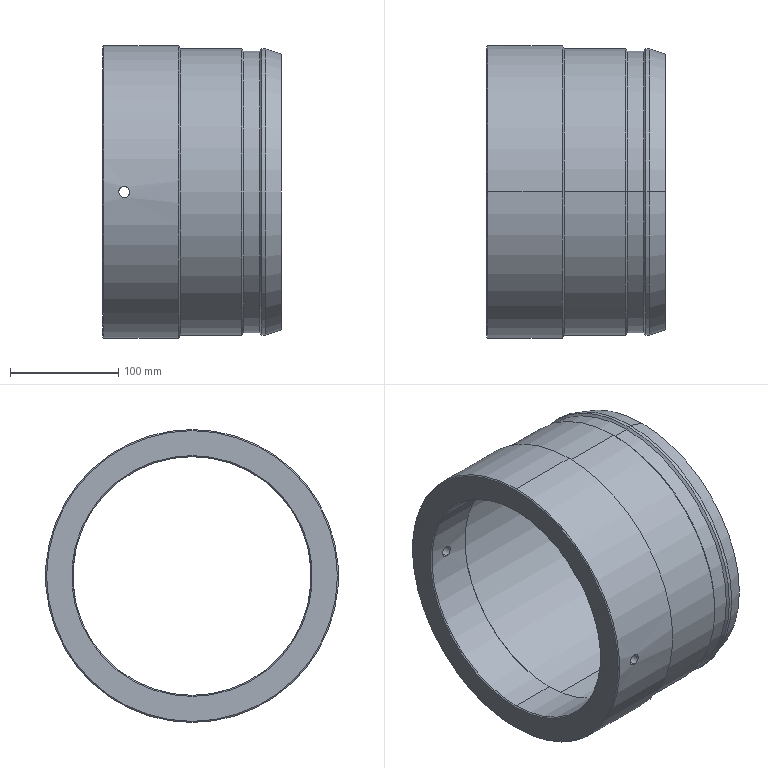Part | SolidWorks | features 3DProfileFeature 1, Chamfer 1, Fillet 1, HoleWzd 1, Revolution 1 | 1 solid | 35 faces | box 165 x 270 x 270 mm | volume 1639814 mm3 | cylinder 16 | cone 14 | plane 3 | torus 2 | commonest cylinder face diameters 10.2 x4 264 x4 220 x2 248 x2 260 x2 270 x2
STEP:
#1=CARTESIAN_POINT('',(20.,-134.904,-5.1));
#2=VERTEX_POINT('',#1);
#3=CARTESIAN_POINT('',(20.,-134.904,5.1));
#4=VERTEX_POINT('',#3);
#5=CARTESIAN_POINT('',(20.,-134.904,-5.1));
#6=CARTESIAN_POINT('',(19.664,-134.904,-5.1));
#7=CARTESIAN_POINT('',(19.331,-134.905,-5.067));
#8=CARTESIAN_POINT('',(18.842,-134.909,-4.97));
#9=CARTESIAN_POINT('',(18.681,-134.91,-4.929));
#10=CARTESIAN_POINT('',(18.361,-134.913,-4.832));
#11=CARTESIAN_POINT('',(18.202,-134.916,-4.775));
#12=CARTESIAN_POINT('',(17.738,-134.922,-4.583));
#13=CARTESIAN_POINT('',(17.445,-134.928,-4.426));
#14=CARTESIAN_POINT('',(16.891,-134.939,-4.057));
#15=CARTESIAN_POINT('',(16.629,-134.946,-3.841));
#16=CARTESIAN_POINT('',(16.158,-134.958,-3.371));
#17=CARTESIAN_POINT('',(15.947,-134.964,-3.114));
#18=CARTESIAN_POINT('',(15.668,-134.973,-2.696));
#19=CARTESIAN_POINT('',(15.581,-134.976,-2.551));
#20=CARTESIAN_POINT('',(15.423,-134.981,-2.257));
#21=CARTESIAN_POINT('',(15.352,-134.984,-2.106));
#22=CARTESIAN_POINT('',(15.162,-134.99,-1.646));
#23=CARTESIAN_POINT('',(15.064,-134.994,-1.326));
#24=CARTESIAN_POINT('',(14.933,-134.999,-0.6664));
#25=CARTESIAN_POINT('',(14.9,-135.,-0.3329));
#26=CARTESIAN_POINT('',(14.9,-135.,0.3408));
#27=CARTESIAN_POINT('',(14.934,-134.999,0.6721));
#28=CARTESIAN_POINT('',(15.031,-134.995,1.161));
#29=CARTESIAN_POINT('',(15.072,-134.994,1.322));
#30=CARTESIAN_POINT('',(15.169,-134.99,1.643));
#31=CARTESIAN_POINT('',(15.226,-134.988,1.802));
#32=CARTESIAN_POINT('',(15.418,-134.981,2.265));
#33=CARTESIAN_POINT('',(15.575,-134.976,2.558));
#34=CARTESIAN_POINT('',(15.946,-134.964,3.112));
#35=CARTESIAN_POINT('',(16.161,-134.958,3.374));
#36=CARTESIAN_POINT('',(16.632,-134.945,3.844));
#37=CARTESIAN_POINT('',(16.889,-134.939,4.055));
#38=CARTESIAN_POINT('',(17.446,-134.928,4.427));
#39=CARTESIAN_POINT('',(17.743,-134.922,4.585));
#40=CARTESIAN_POINT('',(18.357,-134.913,4.839));
#41=CARTESIAN_POINT('',(18.678,-134.91,4.937));
#42=CARTESIAN_POINT('',(19.337,-134.905,5.068));
#43=CARTESIAN_POINT('',(19.667,-134.904,5.1));
#44=CARTESIAN_POINT('',(20.,-134.904,5.1));
#45=B_SPLINE_CURVE_WITH_KNOTS('',3,(#5,#6,#7,#8,#9,#10,#11,#12,#13,#14,#15,#16,#17,#18,#19,#20,#21,#22,#23,#24,#25,#26,#27,#28,#29,#30,#31,#32,#33,#34,#35,#36,#37,#38,#39,#40,#41,#42,#43,#44),.UNSPECIFIED.,.F.,.F.,(4,2,2,2,2,2,2,2,2,2,2,2,2,2,2,2,2,2,2,4),(0.02392,0.02492,0.02542,0.02591,0.02691,0.02791,0.0289,0.0294,0.0299,0.0309,0.03189,0.03289,0.03339,0.03389,0.03488,0.03588,0.03687,0.03787,0.03887,0.03986),.UNSPECIFIED.);
#46=EDGE_CURVE('',#2,#4,#45,.T.);
#47=ORIENTED_EDGE('',*,*,#46,.F.);
#48=CARTESIAN_POINT('',(20.,-109.882,-5.1));
#49=VERTEX_POINT('',#48);
#50=CARTESIAN_POINT('',(20.,135.,-5.1));
#51=DIRECTION('',(0.,1.,0.));
#52=VECTOR('',#51,1000.);
#53=LINE('',#50,#52);
#54=EDGE_CURVE('',#2,#49,#53,.T.);
#55=ORIENTED_EDGE('',*,*,#54,.T.);
#56=CARTESIAN_POINT('',(20.,-109.882,5.1));
#57=VERTEX_POINT('',#56);
#58=CARTESIAN_POINT('',(20.,-109.882,5.1));
#59=CARTESIAN_POINT('',(19.663,-109.882,5.1));
#60=CARTESIAN_POINT('',(19.332,-109.883,5.067));
#61=CARTESIAN_POINT('',(18.843,-109.888,4.97));
#62=CARTESIAN_POINT('',(18.681,-109.89,4.929));
#63=CARTESIAN_POINT('',(18.361,-109.894,4.832));
#64=CARTESIAN_POINT('',(18.201,-109.896,4.775));
#65=CARTESIAN_POINT('',(17.738,-109.905,4.583));
#66=CARTESIAN_POINT('',(17.445,-109.911,4.426));
#67=CARTESIAN_POINT('',(16.891,-109.925,4.056));
#68=CARTESIAN_POINT('',(16.628,-109.933,3.841));
#69=CARTESIAN_POINT('',(16.158,-109.949,3.37));
#70=CARTESIAN_POINT('',(15.947,-109.956,3.114));
#71=CARTESIAN_POINT('',(15.574,-109.971,2.556));
#72=CARTESIAN_POINT('',(15.416,-109.977,2.259));
#73=CARTESIAN_POINT('',(15.161,-109.988,1.645));
#74=CARTESIAN_POINT('',(15.063,-109.993,1.324));
#75=CARTESIAN_POINT('',(14.932,-109.998,0.6655));
#76=CARTESIAN_POINT('',(14.9,-110.,0.3345));
#77=CARTESIAN_POINT('',(14.9,-110.,-0.3309));
#78=CARTESIAN_POINT('',(14.933,-109.998,-0.6688));
#79=CARTESIAN_POINT('',(15.063,-109.993,-1.323));
#80=CARTESIAN_POINT('',(15.16,-109.988,-1.641));
#81=CARTESIAN_POINT('',(15.351,-109.98,-2.104));
#82=CARTESIAN_POINT('',(15.424,-109.977,-2.257));
#83=CARTESIAN_POINT('',(15.581,-109.97,-2.552));
#84=CARTESIAN_POINT('',(15.667,-109.967,-2.695));
#85=CARTESIAN_POINT('',(15.944,-109.956,-3.11));
#86=CARTESIAN_POINT('',(16.155,-109.949,-3.367));
#87=CARTESIAN_POINT('',(16.631,-109.933,-3.844));
#88=CARTESIAN_POINT('',(16.889,-109.925,-4.055));
#89=CARTESIAN_POINT('',(17.303,-109.915,-4.332));
#90=CARTESIAN_POINT('',(17.446,-109.911,-4.418));
#91=CARTESIAN_POINT('',(17.741,-109.905,-4.575));
#92=CARTESIAN_POINT('',(17.894,-109.902,-4.648));
#93=CARTESIAN_POINT('',(18.358,-109.894,-4.84));
#94=CARTESIAN_POINT('',(18.675,-109.889,-4.936));
#95=CARTESIAN_POINT('',(19.329,-109.883,-5.067));
#96=CARTESIAN_POINT('',(19.667,-109.882,-5.1));
#97=CARTESIAN_POINT('',(20.,-109.882,-5.1));
#98=B_SPLINE_CURVE_WITH_KNOTS('',3,(#58,#59,#60,#61,#62,#63,#64,#65,#66,#67,#68,#69,#70,#71,#72,#73,#74,#75,#76,#77,#78,#79,#80,#81,#82,#83,#84,#85,#86,#87,#88,#89,#90,#91,#92,#93,#94,#95,#96,#97),.UNSPECIFIED.,.F.,.F.,(4,2,2,2,2,2,2,2,2,2,2,2,2,2,2,2,2,2,2,4),(0.,0.0009967,0.001495,0.001993,0.00299,0.003987,0.004983,0.00598,0.006977,0.007974,0.00897,0.009967,0.01047,0.01096,0.01196,0.01296,0.01346,0.01395,0.01495,0.01595),.UNSPECIFIED.);
#99=EDGE_CURVE('',#57,#49,#98,.T.);
#100=ORIENTED_EDGE('',*,*,#99,.F.);
#101=CARTESIAN_POINT('',(20.,135.,5.1));
#102=DIRECTION('',(0.,1.,0.));
#103=VECTOR('',#102,1000.);
#104=LINE('',#101,#103);
#105=EDGE_CURVE('',#4,#57,#104,.T.);
#106=ORIENTED_EDGE('',*,*,#105,.F.);
#107=EDGE_LOOP('',(#47,#55,#100,#106));
#108=FACE_OUTER_BOUND('',#107,.T.);
#109=CARTESIAN_POINT('',(20.,135.,0.));
#110=DIRECTION('',(0.,1.,0.));
#111=DIRECTION('',(0.,0.,1.));
#112=AXIS2_PLACEMENT_3D('',#109,#110,#111);
#113=CYLINDRICAL_SURFACE('',#112,5.1);
#114=ADVANCED_FACE('',(#108),#113,.F.);
#115=CARTESIAN_POINT('',(20.,109.882,-5.1));
#116=VERTEX_POINT('',#115);
#117=CARTESIAN_POINT('',(20.,109.882,5.1));
#118=VERTEX_POINT('',#117);
#119=CARTESIAN_POINT('',(20.,109.882,-5.1));
#120=CARTESIAN_POINT('',(19.667,109.882,-5.1));
#121=CARTESIAN_POINT('',(19.336,109.883,-5.068));
#122=CARTESIAN_POINT('',(18.679,109.889,-4.937));
#123=CARTESIAN_POINT('',(18.357,109.894,-4.839));
#124=CARTESIAN_POINT('',(17.743,109.904,-4.585));
#125=CARTESIAN_POINT('',(17.447,109.911,-4.428));
#126=CARTESIAN_POINT('',(16.888,109.925,-4.055));
#127=CARTESIAN_POINT('',(16.632,109.933,-3.844));
#128=CARTESIAN_POINT('',(16.161,109.948,-3.374));
#129=CARTESIAN_POINT('',(15.946,109.956,-3.112));
#130=CARTESIAN_POINT('',(15.575,109.971,-2.557));
#131=CARTESIAN_POINT('',(15.418,109.977,-2.265));
#132=CARTESIAN_POINT('',(15.162,109.988,-1.648));
#133=CARTESIAN_POINT('',(15.064,109.993,-1.324));
#134=CARTESIAN_POINT('',(14.934,109.998,-0.6717));
#135=CARTESIAN_POINT('',(14.9,110.,-0.3406));
#136=CARTESIAN_POINT('',(14.9,110.,0.3322));
#137=CARTESIAN_POINT('',(14.933,109.998,0.6648));
#138=CARTESIAN_POINT('',(15.029,109.994,1.154));
#139=CARTESIAN_POINT('',(15.07,109.992,1.315));
#140=CARTESIAN_POINT('',(15.166,109.988,1.635));
#141=CARTESIAN_POINT('',(15.223,109.985,1.794));
#142=CARTESIAN_POINT('',(15.415,109.977,2.258));
#143=CARTESIAN_POINT('',(15.572,109.971,2.551));
#144=CARTESIAN_POINT('',(15.941,109.957,3.106));
#145=CARTESIAN_POINT('',(16.156,109.949,3.368));
#146=CARTESIAN_POINT('',(16.626,109.933,3.839));
#147=CARTESIAN_POINT('',(16.883,109.926,4.05));
#148=CARTESIAN_POINT('',(17.3,109.915,4.33));
#149=CARTESIAN_POINT('',(17.445,109.911,4.417));
#150=CARTESIAN_POINT('',(17.74,109.905,4.575));
#151=CARTESIAN_POINT('',(17.89,109.902,4.646));
#152=CARTESIAN_POINT('',(18.35,109.894,4.837));
#153=CARTESIAN_POINT('',(18.67,109.889,4.935));
#154=CARTESIAN_POINT('',(19.33,109.883,5.067));
#155=CARTESIAN_POINT('',(19.663,109.882,5.1));
#156=CARTESIAN_POINT('',(20.,109.882,5.1));
#157=B_SPLINE_CURVE_WITH_KNOTS('',3,(#119,#120,#121,#122,#123,#124,#125,#126,#127,#128,#129,#130,#131,#132,#133,#134,#135,#136,#137,#138,#139,#140,#141,#142,#143,#144,#145,#146,#147,#148,#149,#150,#151,#152,#153,#154,#155,#156),.UNSPECIFIED.,.F.,.F.,(4,2,2,2,2,2,2,2,2,2,2,2,2,2,2,2,2,2,4),(0.01595,0.01694,0.01794,0.01894,0.01993,0.02093,0.02193,0.02292,0.02392,0.02492,0.02541,0.02591,0.02691,0.0279,0.0289,0.0294,0.0299,0.03089,0.03189),.UNSPECIFIED.);
#158=EDGE_CURVE('',#116,#118,#157,.T.);
#159=ORIENTED_EDGE('',*,*,#158,.F.);
#160=CARTESIAN_POINT('',(20.,134.904,-5.1));
#161=VERTEX_POINT('',#160);
#162=CARTESIAN_POINT('',(20.,135.,-5.1));
#163=DIRECTION('',(0.,1.,0.));
#164=VECTOR('',#163,1000.);
#165=LINE('',#162,#164);
#166=EDGE_CURVE('',#116,#161,#165,.T.);
#167=ORIENTED_EDGE('',*,*,#166,.T.);
#168=CARTESIAN_POINT('',(20.,134.904,5.1));
#169=VERTEX_POINT('',#168);
#170=CARTESIAN_POINT('',(20.,134.904,5.1));
#171=CARTESIAN_POINT('',(19.663,134.904,5.1));
#172=CARTESIAN_POINT('',(19.332,134.905,5.067));
#173=CARTESIAN_POINT('',(18.843,134.908,4.97));
#174=CARTESIAN_POINT('',(18.681,134.91,4.929));
#175=CARTESIAN_POINT('',(18.361,134.913,4.832));
#176=CARTESIAN_POINT('',(18.201,134.916,4.775));
#177=CARTESIAN_POINT('',(17.738,134.922,4.583));
#178=CARTESIAN_POINT('',(17.445,134.928,4.427));
#179=CARTESIAN_POINT('',(16.891,134.939,4.056));
#180=CARTESIAN_POINT('',(16.628,134.946,3.841));
#181=CARTESIAN_POINT('',(16.158,134.958,3.37));
#182=CARTESIAN_POINT('',(15.947,134.964,3.114));
#183=CARTESIAN_POINT('',(15.574,134.976,2.556));
#184=CARTESIAN_POINT('',(15.416,134.981,2.259));
#185=CARTESIAN_POINT('',(15.161,134.99,1.645));
#186=CARTESIAN_POINT('',(15.063,134.994,1.324));
#187=CARTESIAN_POINT('',(14.932,134.999,0.6654));
#188=CARTESIAN_POINT('',(14.9,135.,0.3345));
#189=CARTESIAN_POINT('',(14.9,135.,-0.3309));
#190=CARTESIAN_POINT('',(14.933,134.999,-0.6688));
#191=CARTESIAN_POINT('',(15.063,134.994,-1.323));
#192=CARTESIAN_POINT('',(15.16,134.99,-1.641));
#193=CARTESIAN_POINT('',(15.351,134.984,-2.104));
#194=CARTESIAN_POINT('',(15.423,134.981,-2.257));
#195=CARTESIAN_POINT('',(15.581,134.976,-2.552));
#196=CARTESIAN_POINT('',(15.667,134.973,-2.695));
#197=CARTESIAN_POINT('',(15.944,134.964,-3.11));
#198=CARTESIAN_POINT('',(16.155,134.958,-3.367));
#199=CARTESIAN_POINT('',(16.631,134.945,-3.844));
#200=CARTESIAN_POINT('',(16.889,134.939,-4.055));
#201=CARTESIAN_POINT('',(17.303,134.931,-4.332));
#202=CARTESIAN_POINT('',(17.446,134.928,-4.418));
#203=CARTESIAN_POINT('',(17.741,134.922,-4.576));
#204=CARTESIAN_POINT('',(17.894,134.92,-4.648));
#205=CARTESIAN_POINT('',(18.358,134.913,-4.84));
#206=CARTESIAN_POINT('',(18.676,134.91,-4.936));
#207=CARTESIAN_POINT('',(19.329,134.905,-5.067));
#208=CARTESIAN_POINT('',(19.667,134.904,-5.1));
#209=CARTESIAN_POINT('',(20.,134.904,-5.1));
#210=B_SPLINE_CURVE_WITH_KNOTS('',3,(#170,#171,#172,#173,#174,#175,#176,#177,#178,#179,#180,#181,#182,#183,#184,#185,#186,#187,#188,#189,#190,#191,#192,#193,#194,#195,#196,#197,#198,#199,#200,#201,#202,#203,#204,#205,#206,#207,#208,#209),.UNSPECIFIED.,.F.,.F.,(4,2,2,2,2,2,2,2,2,2,2,2,2,2,2,2,2,2,2,4),(0.,0.0009966,0.001495,0.001993,0.00299,0.003987,0.004983,0.00598,0.006977,0.007973,0.00897,0.009966,0.01046,0.01096,0.01196,0.01296,0.01345,0.01395,0.01495,0.01595),.UNSPECIFIED.);
#211=EDGE_CURVE('',#169,#161,#210,.T.);
#212=ORIENTED_EDGE('',*,*,#211,.F.);
#213=CARTESIAN_POINT('',(20.,135.,5.1));
#214=DIRECTION('',(0.,1.,0.));
#215=VECTOR('',#214,1000.);
#216=LINE('',#213,#215);
#217=EDGE_CURVE('',#118,#169,#216,.T.);
#218=ORIENTED_EDGE('',*,*,#217,.F.);
#219=EDGE_LOOP('',(#159,#167,#212,#218));
#220=FACE_OUTER_BOUND('',#219,.T.);
#221=CARTESIAN_POINT('',(20.,135.,0.));
#222=DIRECTION('',(0.,1.,0.));
#223=DIRECTION('',(0.,0.,1.));
#224=AXIS2_PLACEMENT_3D('',#221,#222,#223);
#225=CYLINDRICAL_SURFACE('',#224,5.1);
#226=ADVANCED_FACE('',(#220),#225,.F.);
#227=CARTESIAN_POINT('',(0.,0.,134.));
#228=VERTEX_POINT('',#227);
#229=CARTESIAN_POINT('',(0.,0.,-134.));
#230=VERTEX_POINT('',#229);
#231=CARTESIAN_POINT('',(0.,0.,0.));
#232=DIRECTION('',(-1.,0.,0.));
#233=DIRECTION('',(0.,0.,-1.));
#234=AXIS2_PLACEMENT_3D('',#231,#232,#233);
#235=CIRCLE('',#234,134.);
#236=EDGE_CURVE('',#228,#230,#235,.T.);
#237=ORIENTED_EDGE('',*,*,#236,.F.);
#238=CARTESIAN_POINT('',(1.,0.,135.));
#239=VERTEX_POINT('',#238);
#240=CARTESIAN_POINT('',(0.,0.,134.));
#241=DIRECTION('',(0.7071,0.,0.7071));
#242=VECTOR('',#241,1000.);
#243=LINE('',#240,#242);
#244=EDGE_CURVE('',#228,#239,#243,.T.);
#245=ORIENTED_EDGE('',*,*,#244,.T.);
#246=CARTESIAN_POINT('',(1.,0.,-135.));
#247=VERTEX_POINT('',#246);
#248=CARTESIAN_POINT('',(1.,0.,0.));
#249=DIRECTION('',(1.,0.,0.));
#250=DIRECTION('',(0.,0.,-1.));
#251=AXIS2_PLACEMENT_3D('',#248,#249,#250);
#252=CIRCLE('',#251,135.);
#253=EDGE_CURVE('',#247,#239,#252,.T.);
#254=ORIENTED_EDGE('',*,*,#253,.F.);
#255=CARTESIAN_POINT('',(0.,0.,-134.));
#256=DIRECTION('',(0.7071,0.,-0.7071));
#257=VECTOR('',#256,1000.);
#258=LINE('',#255,#257);
#259=EDGE_CURVE('',#230,#247,#258,.T.);
#260=ORIENTED_EDGE('',*,*,#259,.F.);
#261=EDGE_LOOP('',(#237,#245,#254,#260));
#262=FACE_OUTER_BOUND('',#261,.T.);
#263=CARTESIAN_POINT('',(0.,0.,0.));
#264=DIRECTION('',(1.,0.,0.));
#265=DIRECTION('',(0.,0.,-1.));
#266=AXIS2_PLACEMENT_3D('',#263,#264,#265);
#267=CONICAL_SURFACE('',#266,134.,0.7854);
#268=ADVANCED_FACE('',(#262),#267,.T.);
#269=CARTESIAN_POINT('',(1.,0.,-110.));
#270=VERTEX_POINT('',#269);
#271=CARTESIAN_POINT('',(1.,0.,110.));
#272=VERTEX_POINT('',#271);
#273=CARTESIAN_POINT('',(1.,0.,0.));
#274=DIRECTION('',(-1.,0.,0.));
#275=DIRECTION('',(0.,0.,-1.));
#276=AXIS2_PLACEMENT_3D('',#273,#274,#275);
#277=CIRCLE('',#276,110.);
#278=EDGE_CURVE('',#270,#272,#277,.T.);
#279=ORIENTED_EDGE('',*,*,#278,.F.);
#280=CARTESIAN_POINT('',(0.,0.,-111.));
#281=VERTEX_POINT('',#280);
#282=CARTESIAN_POINT('',(1.,0.,-110.));
#283=DIRECTION('',(-0.7071,0.,-0.7071));
#284=VECTOR('',#283,1000.);
#285=LINE('',#282,#284);
#286=EDGE_CURVE('',#270,#281,#285,.T.);
#287=ORIENTED_EDGE('',*,*,#286,.T.);
#288=CARTESIAN_POINT('',(0.,0.,111.));
#289=VERTEX_POINT('',#288);
#290=CARTESIAN_POINT('',(0.,0.,0.));
#291=DIRECTION('',(1.,0.,0.));
#292=DIRECTION('',(0.,0.,-1.));
#293=AXIS2_PLACEMENT_3D('',#290,#291,#292);
#294=CIRCLE('',#293,111.);
#295=EDGE_CURVE('',#289,#281,#294,.T.);
#296=ORIENTED_EDGE('',*,*,#295,.F.);
#297=CARTESIAN_POINT('',(1.,0.,110.));
#298=DIRECTION('',(-0.7071,0.,0.7071));
#299=VECTOR('',#298,1000.);
#300=LINE('',#297,#299);
#301=EDGE_CURVE('',#272,#289,#300,.T.);
#302=ORIENTED_EDGE('',*,*,#301,.F.);
#303=EDGE_LOOP('',(#279,#287,#296,#302));
#304=FACE_OUTER_BOUND('',#303,.T.);
#305=CARTESIAN_POINT('',(1.,0.,0.));
#306=DIRECTION('',(-1.,0.,0.));
#307=DIRECTION('',(0.,0.,1.));
#308=AXIS2_PLACEMENT_3D('',#305,#306,#307);
#309=CONICAL_SURFACE('',#308,110.,0.7854);
#310=ADVANCED_FACE('',(#304),#309,.F.);
#311=CARTESIAN_POINT('',(44.,0.,110.));
#312=VERTEX_POINT('',#311);
#313=CARTESIAN_POINT('',(44.,0.,-110.));
#314=VERTEX_POINT('',#313);
#315=CARTESIAN_POINT('',(44.,0.,0.));
#316=DIRECTION('',(1.,0.,0.));
#317=DIRECTION('',(0.,0.,1.));
#318=AXIS2_PLACEMENT_3D('',#315,#316,#317);
#319=CIRCLE('',#318,110.);
#320=EDGE_CURVE('',#312,#314,#319,.T.);
#321=ORIENTED_EDGE('',*,*,#320,.F.);
#322=CARTESIAN_POINT('',(45.,0.,111.));
#323=VERTEX_POINT('',#322);
#324=CARTESIAN_POINT('',(45.,0.,111.));
#325=DIRECTION('',(0.7071,0.,0.7071));
#326=VECTOR('',#325,1000.);
#327=LINE('',#324,#326);
#328=EDGE_CURVE('',#312,#323,#327,.T.);
#329=ORIENTED_EDGE('',*,*,#328,.T.);
#330=CARTESIAN_POINT('',(45.,0.,-111.));
#331=VERTEX_POINT('',#330);
#332=CARTESIAN_POINT('',(45.,0.,0.));
#333=DIRECTION('',(-1.,0.,0.));
#334=DIRECTION('',(0.,0.,1.));
#335=AXIS2_PLACEMENT_3D('',#332,#333,#334);
#336=CIRCLE('',#335,111.);
#337=EDGE_CURVE('',#331,#323,#336,.T.);
#338=ORIENTED_EDGE('',*,*,#337,.F.);
#339=CARTESIAN_POINT('',(45.,0.,-111.));
#340=DIRECTION('',(0.7071,0.,-0.7071));
#341=VECTOR('',#340,1000.);
#342=LINE('',#339,#341);
#343=EDGE_CURVE('',#314,#331,#342,.T.);
#344=ORIENTED_EDGE('',*,*,#343,.F.);
#345=EDGE_LOOP('',(#321,#329,#338,#344));
#346=FACE_OUTER_BOUND('',#345,.T.);
#347=CARTESIAN_POINT('',(45.,0.,0.));
#348=DIRECTION('',(1.,0.,0.));
#349=DIRECTION('',(0.,0.,-1.));
#350=AXIS2_PLACEMENT_3D('',#347,#348,#349);
#351=CONICAL_SURFACE('',#350,111.,0.7854);
#352=ADVANCED_FACE('',(#346),#351,.F.);
#353=CARTESIAN_POINT('',(47.,0.,-124.));
#354=VERTEX_POINT('',#353);
#355=CARTESIAN_POINT('',(47.,0.,124.));
#356=VERTEX_POINT('',#355);
#357=CARTESIAN_POINT('',(47.,0.,0.));
#358=DIRECTION('',(-1.,0.,0.));
#359=DIRECTION('',(0.,0.,1.));
#360=AXIS2_PLACEMENT_3D('',#357,#358,#359);
#361=CIRCLE('',#360,124.);
#362=EDGE_CURVE('',#354,#356,#361,.T.);
#363=ORIENTED_EDGE('',*,*,#362,.F.);
#364=CARTESIAN_POINT('',(45.,0.,-122.));
#365=VERTEX_POINT('',#364);
#366=CARTESIAN_POINT('',(47.,0.,-122.));
#367=DIRECTION('',(0.,1.,0.));
#368=DIRECTION('',(0.,0.,1.));
#369=AXIS2_PLACEMENT_3D('',#366,#367,#368);
#370=CIRCLE('',#369,2.);
#371=EDGE_CURVE('',#354,#365,#370,.T.);
#372=ORIENTED_EDGE('',*,*,#371,.T.);
#373=CARTESIAN_POINT('',(45.,0.,122.));
#374=VERTEX_POINT('',#373);
#375=CARTESIAN_POINT('',(45.,0.,0.));
#376=DIRECTION('',(1.,0.,0.));
#377=DIRECTION('',(0.,0.,1.));
#378=AXIS2_PLACEMENT_3D('',#375,#376,#377);
#379=CIRCLE('',#378,122.);
#380=EDGE_CURVE('',#374,#365,#379,.T.);
#381=ORIENTED_EDGE('',*,*,#380,.F.);
#382=CARTESIAN_POINT('',(47.,0.,122.));
#383=DIRECTION('',(0.,-1.,0.));
#384=DIRECTION('',(0.,0.,-1.));
#385=AXIS2_PLACEMENT_3D('',#382,#383,#384);
#386=CIRCLE('',#385,2.);
#387=EDGE_CURVE('',#356,#374,#386,.T.);
#388=ORIENTED_EDGE('',*,*,#387,.F.);
#389=EDGE_LOOP('',(#363,#372,#381,#388));
#390=FACE_OUTER_BOUND('',#389,.T.);
#391=CARTESIAN_POINT('',(47.,0.,0.));
#392=DIRECTION('',(-1.,0.,0.));
#393=DIRECTION('',(0.,0.,1.));
#394=AXIS2_PLACEMENT_3D('',#391,#392,#393);
#395=TOROIDAL_SURFACE('',#394,122.,2.);
#396=ADVANCED_FACE('',(#390),#395,.F.);
#397=ORIENTED_EDGE('',*,*,#211,.T.);
#398=CARTESIAN_POINT('',(20.,134.904,-5.1));
#399=CARTESIAN_POINT('',(20.333,134.904,-5.1));
#400=CARTESIAN_POINT('',(20.664,134.905,-5.068));
#401=CARTESIAN_POINT('',(21.321,134.91,-4.937));
#402=CARTESIAN_POINT('',(21.643,134.913,-4.839));
#403=CARTESIAN_POINT('',(22.257,134.922,-4.585));
#404=CARTESIAN_POINT('',(22.553,134.927,-4.428));
#405=CARTESIAN_POINT('',(23.112,134.939,-4.055));
#406=CARTESIAN_POINT('',(23.368,134.945,-3.844));
#407=CARTESIAN_POINT('',(23.839,134.958,-3.374));
#408=CARTESIAN_POINT('',(24.054,134.964,-3.112));
#409=CARTESIAN_POINT('',(24.425,134.976,-2.557));
#410=CARTESIAN_POINT('',(24.582,134.981,-2.264));
#411=CARTESIAN_POINT('',(24.838,134.99,-1.648));
#412=CARTESIAN_POINT('',(24.936,134.994,-1.324));
#413=CARTESIAN_POINT('',(25.066,134.999,-0.6716));
#414=CARTESIAN_POINT('',(25.1,135.,-0.3406));
#415=CARTESIAN_POINT('',(25.1,135.,0.3321));
#416=CARTESIAN_POINT('',(25.067,134.999,0.6648));
#417=CARTESIAN_POINT('',(24.971,134.995,1.154));
#418=CARTESIAN_POINT('',(24.93,134.994,1.315));
#419=CARTESIAN_POINT('',(24.834,134.99,1.635));
#420=CARTESIAN_POINT('',(24.777,134.988,1.794));
#421=CARTESIAN_POINT('',(24.585,134.981,2.258));
#422=CARTESIAN_POINT('',(24.429,134.976,2.551));
#423=CARTESIAN_POINT('',(24.059,134.965,3.105));
#424=CARTESIAN_POINT('',(23.844,134.958,3.368));
#425=CARTESIAN_POINT('',(23.374,134.946,3.839));
#426=CARTESIAN_POINT('',(23.117,134.939,4.05));
#427=CARTESIAN_POINT('',(22.7,134.931,4.33));
#428=CARTESIAN_POINT('',(22.555,134.928,4.417));
#429=CARTESIAN_POINT('',(22.26,134.922,4.575));
#430=CARTESIAN_POINT('',(22.11,134.92,4.646));
#431=CARTESIAN_POINT('',(21.65,134.913,4.837));
#432=CARTESIAN_POINT('',(21.33,134.91,4.935));
#433=CARTESIAN_POINT('',(20.67,134.905,5.067));
#434=CARTESIAN_POINT('',(20.337,134.904,5.1));
#435=CARTESIAN_POINT('',(20.,134.904,5.1));
#436=B_SPLINE_CURVE_WITH_KNOTS('',3,(#398,#399,#400,#401,#402,#403,#404,#405,#406,#407,#408,#409,#410,#411,#412,#413,#414,#415,#416,#417,#418,#419,#420,#421,#422,#423,#424,#425,#426,#427,#428,#429,#430,#431,#432,#433,#434,#435),.UNSPECIFIED.,.F.,.F.,(4,2,2,2,2,2,2,2,2,2,2,2,2,2,2,2,2,2,4),(0.01595,0.01694,0.01794,0.01894,0.01993,0.02093,0.02192,0.02292,0.02392,0.02491,0.02541,0.02591,0.02691,0.0279,0.0289,0.0294,0.0299,0.03089,0.03189),.UNSPECIFIED.);
#437=EDGE_CURVE('',#161,#169,#436,.T.);
#438=ORIENTED_EDGE('',*,*,#437,.T.);
#439=EDGE_LOOP('',(#397,#438));
#440=FACE_BOUND('',#439,.T.);
#441=CARTESIAN_POINT('',(70.,0.,135.));
#442=VERTEX_POINT('',#441);
#443=CARTESIAN_POINT('',(70.,0.,-135.));
#444=VERTEX_POINT('',#443);
#445=CARTESIAN_POINT('',(70.,0.,0.));
#446=DIRECTION('',(-1.,0.,0.));
#447=DIRECTION('',(0.,0.,1.));
#448=AXIS2_PLACEMENT_3D('',#445,#446,#447);
#449=CIRCLE('',#448,135.);
#450=EDGE_CURVE('',#442,#444,#449,.T.);
#451=ORIENTED_EDGE('',*,*,#450,.T.);
#452=CARTESIAN_POINT('',(0.,0.,-135.));
#453=DIRECTION('',(-1.,0.,0.));
#454=VECTOR('',#453,1000.);
#455=LINE('',#452,#454);
#456=EDGE_CURVE('',#444,#247,#455,.T.);
#457=ORIENTED_EDGE('',*,*,#456,.T.);
#458=ORIENTED_EDGE('',*,*,#253,.T.);
#459=CARTESIAN_POINT('',(0.,0.,135.));
#460=DIRECTION('',(-1.,0.,0.));
#461=VECTOR('',#460,1000.);
#462=LINE('',#459,#461);
#463=EDGE_CURVE('',#442,#239,#462,.T.);
#464=ORIENTED_EDGE('',*,*,#463,.F.);
#465=EDGE_LOOP('',(#451,#457,#458,#464));
#466=FACE_OUTER_BOUND('',#465,.T.);
#467=CARTESIAN_POINT('',(0.,0.,0.));
#468=DIRECTION('',(-1.,0.,0.));
#469=DIRECTION('',(0.,0.,1.));
#470=AXIS2_PLACEMENT_3D('',#467,#468,#469);
#471=CYLINDRICAL_SURFACE('',#470,135.);
#472=ADVANCED_FACE('',(#440,#466),#471,.T.);
#473=CARTESIAN_POINT('',(71.732,0.,132.));
#474=VERTEX_POINT('',#473);
#475=CARTESIAN_POINT('',(71.732,0.,-132.));
#476=VERTEX_POINT('',#475);
#477=CARTESIAN_POINT('',(71.732,0.,0.));
#478=DIRECTION('',(-1.,0.,0.));
#479=DIRECTION('',(0.,0.,1.));
#480=AXIS2_PLACEMENT_3D('',#477,#478,#479);
#481=CIRCLE('',#480,132.);
#482=EDGE_CURVE('',#474,#476,#481,.T.);
#483=ORIENTED_EDGE('',*,*,#482,.T.);
#484=CARTESIAN_POINT('',(71.732,0.,-132.));
#485=DIRECTION('',(-0.5,0.,-0.866));
#486=VECTOR('',#485,1000.);
#487=LINE('',#484,#486);
#488=EDGE_CURVE('',#476,#444,#487,.T.);
#489=ORIENTED_EDGE('',*,*,#488,.T.);
#490=ORIENTED_EDGE('',*,*,#450,.F.);
#491=CARTESIAN_POINT('',(71.732,0.,132.));
#492=DIRECTION('',(-0.5,0.,0.866));
#493=VECTOR('',#492,1000.);
#494=LINE('',#491,#493);
#495=EDGE_CURVE('',#474,#442,#494,.T.);
#496=ORIENTED_EDGE('',*,*,#495,.F.);
#497=EDGE_LOOP('',(#483,#489,#490,#496));
#498=FACE_OUTER_BOUND('',#497,.T.);
#499=CARTESIAN_POINT('',(71.732,0.,0.));
#500=DIRECTION('',(-1.,0.,0.));
#501=DIRECTION('',(0.,0.,1.));
#502=AXIS2_PLACEMENT_3D('',#499,#500,#501);
#503=CONICAL_SURFACE('',#502,132.,1.047);
#504=ADVANCED_FACE('',(#498),#503,.T.);
#505=CARTESIAN_POINT('',(128.,0.,132.));
#506=VERTEX_POINT('',#505);
#507=CARTESIAN_POINT('',(128.,0.,-132.));
#508=VERTEX_POINT('',#507);
#509=CARTESIAN_POINT('',(128.,0.,0.));
#510=DIRECTION('',(-1.,0.,0.));
#511=DIRECTION('',(0.,0.,1.));
#512=AXIS2_PLACEMENT_3D('',#509,#510,#511);
#513=CIRCLE('',#512,132.);
#514=EDGE_CURVE('',#506,#508,#513,.T.);
#515=ORIENTED_EDGE('',*,*,#514,.T.);
#516=CARTESIAN_POINT('',(0.,0.,-132.));
#517=DIRECTION('',(-1.,0.,0.));
#518=VECTOR('',#517,1000.);
#519=LINE('',#516,#518);
#520=EDGE_CURVE('',#508,#476,#519,.T.);
#521=ORIENTED_EDGE('',*,*,#520,.T.);
#522=ORIENTED_EDGE('',*,*,#482,.F.);
#523=CARTESIAN_POINT('',(0.,0.,132.));
#524=DIRECTION('',(-1.,0.,0.));
#525=VECTOR('',#524,1000.);
#526=LINE('',#523,#525);
#527=EDGE_CURVE('',#506,#474,#526,.T.);
#528=ORIENTED_EDGE('',*,*,#527,.F.);
#529=EDGE_LOOP('',(#515,#521,#522,#528));
#530=FACE_OUTER_BOUND('',#529,.T.);
#531=CARTESIAN_POINT('',(0.,0.,0.));
#532=DIRECTION('',(-1.,0.,0.));
#533=DIRECTION('',(0.,0.,1.));
#534=AXIS2_PLACEMENT_3D('',#531,#532,#533);
#535=CYLINDRICAL_SURFACE('',#534,132.);
#536=ADVANCED_FACE('',(#530),#535,.T.);
#537=CARTESIAN_POINT('',(130.,0.,130.));
#538=VERTEX_POINT('',#537);
#539=CARTESIAN_POINT('',(130.,0.,-130.));
#540=VERTEX_POINT('',#539);
#541=CARTESIAN_POINT('',(130.,0.,0.));
#542=DIRECTION('',(-1.,0.,0.));
#543=DIRECTION('',(0.,0.,1.));
#544=AXIS2_PLACEMENT_3D('',#541,#542,#543);
#545=CIRCLE('',#544,130.);
#546=EDGE_CURVE('',#538,#540,#545,.T.);
#547=ORIENTED_EDGE('',*,*,#546,.T.);
#548=CARTESIAN_POINT('',(130.,0.,-130.));
#549=DIRECTION('',(-0.7071,0.,-0.7071));
#550=VECTOR('',#549,1000.);
#551=LINE('',#548,#550);
#552=EDGE_CURVE('',#540,#508,#551,.T.);
#553=ORIENTED_EDGE('',*,*,#552,.T.);
#554=ORIENTED_EDGE('',*,*,#514,.F.);
#555=CARTESIAN_POINT('',(130.,0.,130.));
#556=DIRECTION('',(-0.7071,0.,0.7071));
#557=VECTOR('',#556,1000.);
#558=LINE('',#555,#557);
#559=EDGE_CURVE('',#538,#506,#558,.T.);
#560=ORIENTED_EDGE('',*,*,#559,.F.);
#561=EDGE_LOOP('',(#547,#553,#554,#560));
#562=FACE_OUTER_BOUND('',#561,.T.);
#563=CARTESIAN_POINT('',(130.,0.,0.));
#564=DIRECTION('',(-1.,0.,0.));
#565=DIRECTION('',(0.,0.,1.));
#566=AXIS2_PLACEMENT_3D('',#563,#564,#565);
#567=CONICAL_SURFACE('',#566,130.,0.7854);
#568=ADVANCED_FACE('',(#562),#567,.T.);
#569=CARTESIAN_POINT('',(145.,0.,130.));
#570=VERTEX_POINT('',#569);
#571=CARTESIAN_POINT('',(145.,0.,-130.));
#572=VERTEX_POINT('',#571);
#573=CARTESIAN_POINT('',(145.,0.,0.));
#574=DIRECTION('',(-1.,0.,0.));
#575=DIRECTION('',(0.,0.,1.));
#576=AXIS2_PLACEMENT_3D('',#573,#574,#575);
#577=CIRCLE('',#576,130.);
#578=EDGE_CURVE('',#570,#572,#577,.T.);
#579=ORIENTED_EDGE('',*,*,#578,.T.);
#580=CARTESIAN_POINT('',(0.,0.,-130.));
#581=DIRECTION('',(-1.,0.,0.));
#582=VECTOR('',#581,1000.);
#583=LINE('',#580,#582);
#584=EDGE_CURVE('',#572,#540,#583,.T.);
#585=ORIENTED_EDGE('',*,*,#584,.T.);
#586=ORIENTED_EDGE('',*,*,#546,.F.);
#587=CARTESIAN_POINT('',(0.,0.,130.));
#588=DIRECTION('',(-1.,0.,0.));
#589=VECTOR('',#588,1000.);
#590=LINE('',#587,#589);
#591=EDGE_CURVE('',#570,#538,#590,.T.);
#592=ORIENTED_EDGE('',*,*,#591,.F.);
#593=EDGE_LOOP('',(#579,#585,#586,#592));
#594=FACE_OUTER_BOUND('',#593,.T.);
#595=CARTESIAN_POINT('',(0.,0.,0.));
#596=DIRECTION('',(-1.,0.,0.));
#597=DIRECTION('',(0.,0.,1.));
#598=AXIS2_PLACEMENT_3D('',#595,#596,#597);
#599=CYLINDRICAL_SURFACE('',#598,130.);
#600=ADVANCED_FACE('',(#594),#599,.T.);
#601=ORIENTED_EDGE('',*,*,#578,.F.);
#602=CARTESIAN_POINT('',(147.,0.,132.));
#603=VERTEX_POINT('',#602);
#604=CARTESIAN_POINT('',(147.,0.,132.));
#605=DIRECTION('',(0.7071,0.,0.7071));
#606=VECTOR('',#605,1000.);
#607=LINE('',#604,#606);
#608=EDGE_CURVE('',#570,#603,#607,.T.);
#609=ORIENTED_EDGE('',*,*,#608,.T.);
#610=CARTESIAN_POINT('',(147.,0.,-132.));
#611=VERTEX_POINT('',#610);
#612=CARTESIAN_POINT('',(147.,0.,0.));
#613=DIRECTION('',(-1.,0.,0.));
#614=DIRECTION('',(0.,0.,1.));
#615=AXIS2_PLACEMENT_3D('',#612,#613,#614);
#616=CIRCLE('',#615,132.);
#617=EDGE_CURVE('',#603,#611,#616,.T.);
#618=ORIENTED_EDGE('',*,*,#617,.T.);
#619=CARTESIAN_POINT('',(147.,0.,-132.));
#620=DIRECTION('',(0.7071,0.,-0.7071));
#621=VECTOR('',#620,1000.);
#622=LINE('',#619,#621);
#623=EDGE_CURVE('',#572,#611,#622,.T.);
#624=ORIENTED_EDGE('',*,*,#623,.F.);
#625=EDGE_LOOP('',(#601,#609,#618,#624));
#626=FACE_OUTER_BOUND('',#625,.T.);
#627=CARTESIAN_POINT('',(147.,0.,0.));
#628=DIRECTION('',(1.,0.,0.));
#629=DIRECTION('',(0.,0.,-1.));
#630=AXIS2_PLACEMENT_3D('',#627,#628,#629);
#631=CONICAL_SURFACE('',#630,132.,0.7854);
#632=ADVANCED_FACE('',(#626),#631,.T.);
#633=CARTESIAN_POINT('',(150.,0.,132.));
#634=VERTEX_POINT('',#633);
#635=CARTESIAN_POINT('',(150.,0.,-132.));
#636=VERTEX_POINT('',#635);
#637=CARTESIAN_POINT('',(150.,0.,0.));
#638=DIRECTION('',(-1.,0.,0.));
#639=DIRECTION('',(0.,0.,1.));
#640=AXIS2_PLACEMENT_3D('',#637,#638,#639);
#641=CIRCLE('',#640,132.);
#642=EDGE_CURVE('',#634,#636,#641,.T.);
#643=ORIENTED_EDGE('',*,*,#642,.T.);
#644=CARTESIAN_POINT('',(0.,0.,-132.));
#645=DIRECTION('',(-1.,0.,0.));
#646=VECTOR('',#645,1000.);
#647=LINE('',#644,#646);
#648=EDGE_CURVE('',#636,#611,#647,.T.);
#649=ORIENTED_EDGE('',*,*,#648,.T.);
#650=ORIENTED_EDGE('',*,*,#617,.F.);
#651=CARTESIAN_POINT('',(0.,0.,132.));
#652=DIRECTION('',(-1.,0.,0.));
#653=VECTOR('',#652,1000.);
#654=LINE('',#651,#653);
#655=EDGE_CURVE('',#634,#603,#654,.T.);
#656=ORIENTED_EDGE('',*,*,#655,.F.);
#657=EDGE_LOOP('',(#643,#649,#650,#656));
#658=FACE_OUTER_BOUND('',#657,.T.);
#659=CARTESIAN_POINT('',(0.,0.,0.));
#660=DIRECTION('',(-1.,0.,0.));
#661=DIRECTION('',(0.,0.,1.));
#662=AXIS2_PLACEMENT_3D('',#659,#660,#661);
#663=CYLINDRICAL_SURFACE('',#662,132.);
#664=ADVANCED_FACE('',(#658),#663,.T.);
#665=CARTESIAN_POINT('',(165.,0.,127.));
#666=VERTEX_POINT('',#665);
#667=CARTESIAN_POINT('',(165.,0.,-127.));
#668=VERTEX_POINT('',#667);
#669=CARTESIAN_POINT('',(165.,0.,0.));
#670=DIRECTION('',(-1.,0.,0.));
#671=DIRECTION('',(0.,0.,1.));
#672=AXIS2_PLACEMENT_3D('',#669,#670,#671);
#673=CIRCLE('',#672,127.);
#674=EDGE_CURVE('',#666,#668,#673,.T.);
#675=ORIENTED_EDGE('',*,*,#674,.T.);
#676=CARTESIAN_POINT('',(165.,0.,-127.));
#677=DIRECTION('',(-0.9487,0.,-0.3162));
#678=VECTOR('',#677,1000.);
#679=LINE('',#676,#678);
#680=EDGE_CURVE('',#668,#636,#679,.T.);
#681=ORIENTED_EDGE('',*,*,#680,.T.);
#682=ORIENTED_EDGE('',*,*,#642,.F.);
#683=CARTESIAN_POINT('',(165.,0.,127.));
#684=DIRECTION('',(-0.9487,0.,0.3162));
#685=VECTOR('',#684,1000.);
#686=LINE('',#683,#685);
#687=EDGE_CURVE('',#666,#634,#686,.T.);
#688=ORIENTED_EDGE('',*,*,#687,.F.);
#689=EDGE_LOOP('',(#675,#681,#682,#688));
#690=FACE_OUTER_BOUND('',#689,.T.);
#691=CARTESIAN_POINT('',(165.,0.,0.));
#692=DIRECTION('',(-1.,0.,0.));
#693=DIRECTION('',(0.,0.,1.));
#694=AXIS2_PLACEMENT_3D('',#691,#692,#693);
#695=CONICAL_SURFACE('',#694,127.,0.3218);
#696=ADVANCED_FACE('',(#690),#695,.T.);
#697=CARTESIAN_POINT('',(165.,0.,-124.));
#698=VERTEX_POINT('',#697);
#699=CARTESIAN_POINT('',(165.,0.,124.));
#700=VERTEX_POINT('',#699);
#701=CARTESIAN_POINT('',(165.,0.,0.));
#702=DIRECTION('',(-1.,0.,0.));
#703=DIRECTION('',(0.,0.,1.));
#704=AXIS2_PLACEMENT_3D('',#701,#702,#703);
#705=CIRCLE('',#704,124.);
#706=EDGE_CURVE('',#698,#700,#705,.T.);
#707=ORIENTED_EDGE('',*,*,#706,.F.);
#708=CARTESIAN_POINT('',(0.,0.,-124.));
#709=DIRECTION('',(-1.,0.,0.));
#710=VECTOR('',#709,1000.);
#711=LINE('',#708,#710);
#712=EDGE_CURVE('',#698,#354,#711,.T.);
#713=ORIENTED_EDGE('',*,*,#712,.T.);
#714=ORIENTED_EDGE('',*,*,#362,.T.);
#715=CARTESIAN_POINT('',(0.,0.,124.));
#716=DIRECTION('',(-1.,0.,0.));
#717=VECTOR('',#716,1000.);
#718=LINE('',#715,#717);
#719=EDGE_CURVE('',#700,#356,#718,.T.);
#720=ORIENTED_EDGE('',*,*,#719,.F.);
#721=EDGE_LOOP('',(#707,#713,#714,#720));
#722=FACE_OUTER_BOUND('',#721,.T.);
#723=CARTESIAN_POINT('',(0.,0.,0.));
#724=DIRECTION('',(-1.,0.,0.));
#725=DIRECTION('',(0.,0.,1.));
#726=AXIS2_PLACEMENT_3D('',#723,#724,#725);
#727=CYLINDRICAL_SURFACE('',#726,124.);
#728=ADVANCED_FACE('',(#722),#727,.F.);
#729=ORIENTED_EDGE('',*,*,#99,.T.);
#730=CARTESIAN_POINT('',(20.,-109.882,-5.1));
#731=CARTESIAN_POINT('',(20.333,-109.882,-5.1));
#732=CARTESIAN_POINT('',(20.664,-109.883,-5.068));
#733=CARTESIAN_POINT('',(21.321,-109.889,-4.937));
#734=CARTESIAN_POINT('',(21.643,-109.894,-4.839));
#735=CARTESIAN_POINT('',(22.257,-109.904,-4.585));
#736=CARTESIAN_POINT('',(22.553,-109.911,-4.428));
#737=CARTESIAN_POINT('',(23.112,-109.925,-4.055));
#738=CARTESIAN_POINT('',(23.368,-109.933,-3.844));
#739=CARTESIAN_POINT('',(23.839,-109.948,-3.374));
#740=CARTESIAN_POINT('',(24.054,-109.956,-3.112));
#741=CARTESIAN_POINT('',(24.425,-109.971,-2.557));
#742=CARTESIAN_POINT('',(24.582,-109.977,-2.265));
#743=CARTESIAN_POINT('',(24.838,-109.988,-1.648));
#744=CARTESIAN_POINT('',(24.936,-109.993,-1.324));
#745=CARTESIAN_POINT('',(25.066,-109.998,-0.6717));
#746=CARTESIAN_POINT('',(25.1,-110.,-0.3406));
#747=CARTESIAN_POINT('',(25.1,-110.,0.3322));
#748=CARTESIAN_POINT('',(25.067,-109.998,0.6648));
#749=CARTESIAN_POINT('',(24.971,-109.994,1.154));
#750=CARTESIAN_POINT('',(24.93,-109.992,1.315));
#751=CARTESIAN_POINT('',(24.834,-109.988,1.635));
#752=CARTESIAN_POINT('',(24.777,-109.985,1.794));
#753=CARTESIAN_POINT('',(24.585,-109.977,2.258));
#754=CARTESIAN_POINT('',(24.428,-109.971,2.551));
#755=CARTESIAN_POINT('',(24.059,-109.957,3.106));
#756=CARTESIAN_POINT('',(23.844,-109.949,3.368));
#757=CARTESIAN_POINT('',(23.374,-109.933,3.839));
#758=CARTESIAN_POINT('',(23.117,-109.926,4.05));
#759=CARTESIAN_POINT('',(22.7,-109.915,4.33));
#760=CARTESIAN_POINT('',(22.555,-109.911,4.417));
#761=CARTESIAN_POINT('',(22.26,-109.905,4.575));
#762=CARTESIAN_POINT('',(22.11,-109.902,4.646));
#763=CARTESIAN_POINT('',(21.65,-109.894,4.837));
#764=CARTESIAN_POINT('',(21.33,-109.889,4.935));
#765=CARTESIAN_POINT('',(20.67,-109.883,5.067));
#766=CARTESIAN_POINT('',(20.337,-109.882,5.1));
#767=CARTESIAN_POINT('',(20.,-109.882,5.1));
#768=B_SPLINE_CURVE_WITH_KNOTS('',3,(#730,#731,#732,#733,#734,#735,#736,#737,#738,#739,#740,#741,#742,#743,#744,#745,#746,#747,#748,#749,#750,#751,#752,#753,#754,#755,#756,#757,#758,#759,#760,#761,#762,#763,#764,#765,#766,#767),.UNSPECIFIED.,.F.,.F.,(4,2,2,2,2,2,2,2,2,2,2,2,2,2,2,2,2,2,4),(0.01595,0.01694,0.01794,0.01894,0.01993,0.02093,0.02193,0.02292,0.02392,0.02492,0.02541,0.02591,0.02691,0.0279,0.0289,0.0294,0.0299,0.03089,0.03189),.UNSPECIFIED.);
#769=EDGE_CURVE('',#49,#57,#768,.T.);
#770=ORIENTED_EDGE('',*,*,#769,.T.);
#771=EDGE_LOOP('',(#729,#770));
#772=FACE_BOUND('',#771,.T.);
#773=ORIENTED_EDGE('',*,*,#320,.T.);
#774=CARTESIAN_POINT('',(0.,0.,-110.));
#775=DIRECTION('',(-1.,0.,0.));
#776=VECTOR('',#775,1000.);
#777=LINE('',#774,#776);
#778=EDGE_CURVE('',#314,#270,#777,.T.);
#779=ORIENTED_EDGE('',*,*,#778,.T.);
#780=ORIENTED_EDGE('',*,*,#278,.T.);
#781=CARTESIAN_POINT('',(0.,0.,110.));
#782=DIRECTION('',(-1.,0.,0.));
#783=VECTOR('',#782,1000.);
#784=LINE('',#781,#783);
#785=EDGE_CURVE('',#312,#272,#784,.T.);
#786=ORIENTED_EDGE('',*,*,#785,.F.);
#787=EDGE_LOOP('',(#773,#779,#780,#786));
#788=FACE_OUTER_BOUND('',#787,.T.);
#789=CARTESIAN_POINT('',(0.,0.,0.));
#790=DIRECTION('',(-1.,0.,0.));
#791=DIRECTION('',(0.,0.,1.));
#792=AXIS2_PLACEMENT_3D('',#789,#790,#791);
#793=CYLINDRICAL_SURFACE('',#792,110.);
#794=ADVANCED_FACE('',(#772,#788),#793,.F.);
#795=ORIENTED_EDGE('',*,*,#295,.T.);
#796=CARTESIAN_POINT('',(0.,0.,0.));
#797=DIRECTION('',(1.,0.,0.));
#798=DIRECTION('',(0.,0.,-1.));
#799=AXIS2_PLACEMENT_3D('',#796,#797,#798);
#800=CIRCLE('',#799,111.);
#801=EDGE_CURVE('',#281,#289,#800,.T.);
#802=ORIENTED_EDGE('',*,*,#801,.T.);
#803=EDGE_LOOP('',(#795,#802));
#804=FACE_BOUND('',#803,.T.);
#805=CARTESIAN_POINT('',(0.,0.,0.));
#806=DIRECTION('',(-1.,0.,0.));
#807=DIRECTION('',(0.,0.,-1.));
#808=AXIS2_PLACEMENT_3D('',#805,#806,#807);
#809=CIRCLE('',#808,134.);
#810=EDGE_CURVE('',#230,#228,#809,.T.);
#811=ORIENTED_EDGE('',*,*,#810,.T.);
#812=ORIENTED_EDGE('',*,*,#236,.T.);
#813=EDGE_LOOP('',(#811,#812));
#814=FACE_OUTER_BOUND('',#813,.T.);
#815=CARTESIAN_POINT('',(0.,135.,0.));
#816=DIRECTION('',(1.,0.,0.));
#817=DIRECTION('',(0.,0.,-1.));
#818=AXIS2_PLACEMENT_3D('',#815,#816,#817);
#819=PLANE('',#818);
#820=ADVANCED_FACE('',(#804,#814),#819,.F.);
#821=ORIENTED_EDGE('',*,*,#778,.F.);
#822=CARTESIAN_POINT('',(44.,0.,0.));
#823=DIRECTION('',(1.,0.,0.));
#824=DIRECTION('',(0.,0.,1.));
#825=AXIS2_PLACEMENT_3D('',#822,#823,#824);
#826=CIRCLE('',#825,110.);
#827=EDGE_CURVE('',#314,#312,#826,.T.);
#828=ORIENTED_EDGE('',*,*,#827,.T.);
#829=ORIENTED_EDGE('',*,*,#785,.T.);
#830=CARTESIAN_POINT('',(1.,0.,0.));
#831=DIRECTION('',(-1.,0.,0.));
#832=DIRECTION('',(0.,0.,-1.));
#833=AXIS2_PLACEMENT_3D('',#830,#831,#832);
#834=CIRCLE('',#833,110.);
#835=EDGE_CURVE('',#272,#270,#834,.T.);
#836=ORIENTED_EDGE('',*,*,#835,.T.);
#837=EDGE_LOOP('',(#821,#828,#829,#836));
#838=FACE_OUTER_BOUND('',#837,.T.);
#839=CARTESIAN_POINT('',(20.,109.882,5.1));
#840=CARTESIAN_POINT('',(20.337,109.882,5.1));
#841=CARTESIAN_POINT('',(20.668,109.883,5.067));
#842=CARTESIAN_POINT('',(21.157,109.888,4.97));
#843=CARTESIAN_POINT('',(21.319,109.89,4.929));
#844=CARTESIAN_POINT('',(21.639,109.894,4.832));
#845=CARTESIAN_POINT('',(21.799,109.896,4.775));
#846=CARTESIAN_POINT('',(22.262,109.905,4.583));
#847=CARTESIAN_POINT('',(22.555,109.911,4.426));
#848=CARTESIAN_POINT('',(23.109,109.925,4.056));
#849=CARTESIAN_POINT('',(23.372,109.933,3.841));
#850=CARTESIAN_POINT('',(23.842,109.949,3.37));
#851=CARTESIAN_POINT('',(24.053,109.956,3.114));
#852=CARTESIAN_POINT('',(24.426,109.971,2.556));
#853=CARTESIAN_POINT('',(24.584,109.977,2.259));
#854=CARTESIAN_POINT('',(24.839,109.988,1.645));
#855=CARTESIAN_POINT('',(24.937,109.993,1.324));
#856=CARTESIAN_POINT('',(25.068,109.998,0.6655));
#857=CARTESIAN_POINT('',(25.1,110.,0.3345));
#858=CARTESIAN_POINT('',(25.1,110.,-0.3309));
#859=CARTESIAN_POINT('',(25.067,109.998,-0.6688));
#860=CARTESIAN_POINT('',(24.937,109.993,-1.323));
#861=CARTESIAN_POINT('',(24.84,109.988,-1.641));
#862=CARTESIAN_POINT('',(24.649,109.98,-2.104));
#863=CARTESIAN_POINT('',(24.576,109.977,-2.257));
#864=CARTESIAN_POINT('',(24.419,109.97,-2.552));
#865=CARTESIAN_POINT('',(24.333,109.967,-2.695));
#866=CARTESIAN_POINT('',(24.056,109.956,-3.11));
#867=CARTESIAN_POINT('',(23.845,109.949,-3.367));
#868=CARTESIAN_POINT('',(23.369,109.933,-3.844));
#869=CARTESIAN_POINT('',(23.111,109.925,-4.055));
#870=CARTESIAN_POINT('',(22.697,109.915,-4.332));
#871=CARTESIAN_POINT('',(22.554,109.911,-4.418));
#872=CARTESIAN_POINT('',(22.259,109.905,-4.575));
#873=CARTESIAN_POINT('',(22.106,109.902,-4.648));
#874=CARTESIAN_POINT('',(21.642,109.894,-4.84));
#875=CARTESIAN_POINT('',(21.325,109.889,-4.936));
#876=CARTESIAN_POINT('',(20.671,109.883,-5.067));
#877=CARTESIAN_POINT('',(20.333,109.882,-5.1));
#878=CARTESIAN_POINT('',(20.,109.882,-5.1));
#879=B_SPLINE_CURVE_WITH_KNOTS('',3,(#839,#840,#841,#842,#843,#844,#845,#846,#847,#848,#849,#850,#851,#852,#853,#854,#855,#856,#857,#858,#859,#860,#861,#862,#863,#864,#865,#866,#867,#868,#869,#870,#871,#872,#873,#874,#875,#876,#877,#878),.UNSPECIFIED.,.F.,.F.,(4,2,2,2,2,2,2,2,2,2,2,2,2,2,2,2,2,2,2,4),(0.,0.0009967,0.001495,0.001993,0.00299,0.003987,0.004983,0.00598,0.006977,0.007974,0.00897,0.009967,0.01047,0.01096,0.01196,0.01296,0.01346,0.01395,0.01495,0.01595),.UNSPECIFIED.);
#880=EDGE_CURVE('',#118,#116,#879,.T.);
#881=ORIENTED_EDGE('',*,*,#880,.T.);
#882=ORIENTED_EDGE('',*,*,#158,.T.);
#883=EDGE_LOOP('',(#881,#882));
#884=FACE_BOUND('',#883,.T.);
#885=CARTESIAN_POINT('',(0.,0.,0.));
#886=DIRECTION('',(-1.,0.,0.));
#887=DIRECTION('',(0.,0.,1.));
#888=AXIS2_PLACEMENT_3D('',#885,#886,#887);
#889=CYLINDRICAL_SURFACE('',#888,110.);
#890=ADVANCED_FACE('',(#838,#884),#889,.F.);
#891=ORIENTED_EDGE('',*,*,#337,.T.);
#892=CARTESIAN_POINT('',(45.,0.,0.));
#893=DIRECTION('',(-1.,0.,0.));
#894=DIRECTION('',(0.,0.,1.));
#895=AXIS2_PLACEMENT_3D('',#892,#893,#894);
#896=CIRCLE('',#895,111.);
#897=EDGE_CURVE('',#323,#331,#896,.T.);
#898=ORIENTED_EDGE('',*,*,#897,.T.);
#899=EDGE_LOOP('',(#891,#898));
#900=FACE_BOUND('',#899,.T.);
#901=ORIENTED_EDGE('',*,*,#380,.T.);
#902=CARTESIAN_POINT('',(45.,0.,0.));
#903=DIRECTION('',(1.,0.,0.));
#904=DIRECTION('',(0.,0.,1.));
#905=AXIS2_PLACEMENT_3D('',#902,#903,#904);
#906=CIRCLE('',#905,122.);
#907=EDGE_CURVE('',#365,#374,#906,.T.);
#908=ORIENTED_EDGE('',*,*,#907,.T.);
#909=EDGE_LOOP('',(#901,#908));
#910=FACE_OUTER_BOUND('',#909,.T.);
#911=CARTESIAN_POINT('',(45.,110.,0.));
#912=DIRECTION('',(-1.,0.,0.));
#913=DIRECTION('',(0.,0.,1.));
#914=AXIS2_PLACEMENT_3D('',#911,#912,#913);
#915=PLANE('',#914);
#916=ADVANCED_FACE('',(#900,#910),#915,.F.);
#917=ORIENTED_EDGE('',*,*,#712,.F.);
#918=CARTESIAN_POINT('',(165.,0.,0.));
#919=DIRECTION('',(-1.,0.,0.));
#920=DIRECTION('',(0.,0.,1.));
#921=AXIS2_PLACEMENT_3D('',#918,#919,#920);
#922=CIRCLE('',#921,124.);
#923=EDGE_CURVE('',#700,#698,#922,.T.);
#924=ORIENTED_EDGE('',*,*,#923,.F.);
#925=ORIENTED_EDGE('',*,*,#719,.T.);
#926=CARTESIAN_POINT('',(47.,0.,0.));
#927=DIRECTION('',(-1.,0.,0.));
#928=DIRECTION('',(0.,0.,1.));
#929=AXIS2_PLACEMENT_3D('',#926,#927,#928);
#930=CIRCLE('',#929,124.);
#931=EDGE_CURVE('',#356,#354,#930,.T.);
#932=ORIENTED_EDGE('',*,*,#931,.T.);
#933=EDGE_LOOP('',(#917,#924,#925,#932));
#934=FACE_OUTER_BOUND('',#933,.T.);
#935=CARTESIAN_POINT('',(0.,0.,0.));
#936=DIRECTION('',(-1.,0.,0.));
#937=DIRECTION('',(0.,0.,1.));
#938=AXIS2_PLACEMENT_3D('',#935,#936,#937);
#939=CYLINDRICAL_SURFACE('',#938,124.);
#940=ADVANCED_FACE('',(#934),#939,.F.);
#941=ORIENTED_EDGE('',*,*,#674,.F.);
#942=CARTESIAN_POINT('',(165.,0.,0.));
#943=DIRECTION('',(-1.,0.,0.));
#944=DIRECTION('',(0.,0.,1.));
#945=AXIS2_PLACEMENT_3D('',#942,#943,#944);
#946=CIRCLE('',#945,127.);
#947=EDGE_CURVE('',#668,#666,#946,.T.);
#948=ORIENTED_EDGE('',*,*,#947,.F.);
#949=EDGE_LOOP('',(#941,#948));
#950=FACE_OUTER_BOUND('',#949,.T.);
#951=ORIENTED_EDGE('',*,*,#923,.T.);
#952=ORIENTED_EDGE('',*,*,#706,.T.);
#953=EDGE_LOOP('',(#951,#952));
#954=FACE_BOUND('',#953,.T.);
#955=CARTESIAN_POINT('',(165.,124.,0.));
#956=DIRECTION('',(-1.,0.,0.));
#957=DIRECTION('',(0.,0.,1.));
#958=AXIS2_PLACEMENT_3D('',#955,#956,#957);
#959=PLANE('',#958);
#960=ADVANCED_FACE('',(#950,#954),#959,.F.);
#961=ORIENTED_EDGE('',*,*,#680,.F.);
#962=ORIENTED_EDGE('',*,*,#947,.T.);
#963=ORIENTED_EDGE('',*,*,#687,.T.);
#964=CARTESIAN_POINT('',(150.,0.,0.));
#965=DIRECTION('',(-1.,0.,0.));
#966=DIRECTION('',(0.,0.,1.));
#967=AXIS2_PLACEMENT_3D('',#964,#965,#966);
#968=CIRCLE('',#967,132.);
#969=EDGE_CURVE('',#636,#634,#968,.T.);
#970=ORIENTED_EDGE('',*,*,#969,.F.);
#971=EDGE_LOOP('',(#961,#962,#963,#970));
#972=FACE_OUTER_BOUND('',#971,.T.);
#973=CARTESIAN_POINT('',(165.,0.,0.));
#974=DIRECTION('',(-1.,0.,0.));
#975=DIRECTION('',(0.,0.,1.));
#976=AXIS2_PLACEMENT_3D('',#973,#974,#975);
#977=CONICAL_SURFACE('',#976,127.,0.3218);
#978=ADVANCED_FACE('',(#972),#977,.T.);
#979=ORIENTED_EDGE('',*,*,#648,.F.);
#980=ORIENTED_EDGE('',*,*,#969,.T.);
#981=ORIENTED_EDGE('',*,*,#655,.T.);
#982=CARTESIAN_POINT('',(147.,0.,0.));
#983=DIRECTION('',(-1.,0.,0.));
#984=DIRECTION('',(0.,0.,1.));
#985=AXIS2_PLACEMENT_3D('',#982,#983,#984);
#986=CIRCLE('',#985,132.);
#987=EDGE_CURVE('',#611,#603,#986,.T.);
#988=ORIENTED_EDGE('',*,*,#987,.F.);
#989=EDGE_LOOP('',(#979,#980,#981,#988));
#990=FACE_OUTER_BOUND('',#989,.T.);
#991=CARTESIAN_POINT('',(0.,0.,0.));
#992=DIRECTION('',(-1.,0.,0.));
#993=DIRECTION('',(0.,0.,1.));
#994=AXIS2_PLACEMENT_3D('',#991,#992,#993);
#995=CYLINDRICAL_SURFACE('',#994,132.);
#996=ADVANCED_FACE('',(#990),#995,.T.);
#997=ORIENTED_EDGE('',*,*,#608,.F.);
#998=CARTESIAN_POINT('',(145.,0.,0.));
#999=DIRECTION('',(-1.,0.,0.));
#1000=DIRECTION('',(0.,0.,1.));
#1001=AXIS2_PLACEMENT_3D('',#998,#999,#1000);
#1002=CIRCLE('',#1001,130.);
#1003=EDGE_CURVE('',#572,#570,#1002,.T.);
#1004=ORIENTED_EDGE('',*,*,#1003,.F.);
#1005=ORIENTED_EDGE('',*,*,#623,.T.);
#1006=ORIENTED_EDGE('',*,*,#987,.T.);
#1007=EDGE_LOOP('',(#997,#1004,#1005,#1006));
#1008=FACE_OUTER_BOUND('',#1007,.T.);
#1009=CARTESIAN_POINT('',(147.,0.,0.));
#1010=DIRECTION('',(1.,0.,0.));
#1011=DIRECTION('',(0.,0.,-1.));
#1012=AXIS2_PLACEMENT_3D('',#1009,#1010,#1011);
#1013=CONICAL_SURFACE('',#1012,132.,0.7854);
#1014=ADVANCED_FACE('',(#1008),#1013,.T.);
#1015=ORIENTED_EDGE('',*,*,#584,.F.);
#1016=ORIENTED_EDGE('',*,*,#1003,.T.);
#1017=ORIENTED_EDGE('',*,*,#591,.T.);
#1018=CARTESIAN_POINT('',(130.,0.,0.));
#1019=DIRECTION('',(-1.,0.,0.));
#1020=DIRECTION('',(0.,0.,1.));
#1021=AXIS2_PLACEMENT_3D('',#1018,#1019,#1020);
#1022=CIRCLE('',#1021,130.);
#1023=EDGE_CURVE('',#540,#538,#1022,.T.);
#1024=ORIENTED_EDGE('',*,*,#1023,.F.);
#1025=EDGE_LOOP('',(#1015,#1016,#1017,#1024));
#1026=FACE_OUTER_BOUND('',#1025,.T.);
#1027=CARTESIAN_POINT('',(0.,0.,0.));
#1028=DIRECTION('',(-1.,0.,0.));
#1029=DIRECTION('',(0.,0.,1.));
#1030=AXIS2_PLACEMENT_3D('',#1027,#1028,#1029);
#1031=CYLINDRICAL_SURFACE('',#1030,130.);
#1032=ADVANCED_FACE('',(#1026),#1031,.T.);
#1033=ORIENTED_EDGE('',*,*,#552,.F.);
#1034=ORIENTED_EDGE('',*,*,#1023,.T.);
#1035=ORIENTED_EDGE('',*,*,#559,.T.);
#1036=CARTESIAN_POINT('',(128.,0.,0.));
#1037=DIRECTION('',(-1.,0.,0.));
#1038=DIRECTION('',(0.,0.,1.));
#1039=AXIS2_PLACEMENT_3D('',#1036,#1037,#1038);
#1040=CIRCLE('',#1039,132.);
#1041=EDGE_CURVE('',#508,#506,#1040,.T.);
#1042=ORIENTED_EDGE('',*,*,#1041,.F.);
#1043=EDGE_LOOP('',(#1033,#1034,#1035,#1042));
#1044=FACE_OUTER_BOUND('',#1043,.T.);
#1045=CARTESIAN_POINT('',(130.,0.,0.));
#1046=DIRECTION('',(-1.,0.,0.));
#1047=DIRECTION('',(0.,0.,1.));
#1048=AXIS2_PLACEMENT_3D('',#1045,#1046,#1047);
#1049=CONICAL_SURFACE('',#1048,130.,0.7854);
#1050=ADVANCED_FACE('',(#1044),#1049,.T.);
#1051=ORIENTED_EDGE('',*,*,#520,.F.);
#1052=ORIENTED_EDGE('',*,*,#1041,.T.);
#1053=ORIENTED_EDGE('',*,*,#527,.T.);
#1054=CARTESIAN_POINT('',(71.732,0.,0.));
#1055=DIRECTION('',(-1.,0.,0.));
#1056=DIRECTION('',(0.,0.,1.));
#1057=AXIS2_PLACEMENT_3D('',#1054,#1055,#1056);
#1058=CIRCLE('',#1057,132.);
#1059=EDGE_CURVE('',#476,#474,#1058,.T.);
#1060=ORIENTED_EDGE('',*,*,#1059,.F.);
#1061=EDGE_LOOP('',(#1051,#1052,#1053,#1060));
#1062=FACE_OUTER_BOUND('',#1061,.T.);
#1063=CARTESIAN_POINT('',(0.,0.,0.));
#1064=DIRECTION('',(-1.,0.,0.));
#1065=DIRECTION('',(0.,0.,1.));
#1066=AXIS2_PLACEMENT_3D('',#1063,#1064,#1065);
#1067=CYLINDRICAL_SURFACE('',#1066,132.);
#1068=ADVANCED_FACE('',(#1062),#1067,.T.);
#1069=ORIENTED_EDGE('',*,*,#488,.F.);
#1070=ORIENTED_EDGE('',*,*,#1059,.T.);
#1071=ORIENTED_EDGE('',*,*,#495,.T.);
#1072=CARTESIAN_POINT('',(70.,0.,0.));
#1073=DIRECTION('',(-1.,0.,0.));
#1074=DIRECTION('',(0.,0.,1.));
#1075=AXIS2_PLACEMENT_3D('',#1072,#1073,#1074);
#1076=CIRCLE('',#1075,135.);
#1077=EDGE_CURVE('',#444,#442,#1076,.T.);
#1078=ORIENTED_EDGE('',*,*,#1077,.F.);
#1079=EDGE_LOOP('',(#1069,#1070,#1071,#1078));
#1080=FACE_OUTER_BOUND('',#1079,.T.);
#1081=CARTESIAN_POINT('',(71.732,0.,0.));
#1082=DIRECTION('',(-1.,0.,0.));
#1083=DIRECTION('',(0.,0.,1.));
#1084=AXIS2_PLACEMENT_3D('',#1081,#1082,#1083);
#1085=CONICAL_SURFACE('',#1084,132.,1.047);
#1086=ADVANCED_FACE('',(#1080),#1085,.T.);
#1087=ORIENTED_EDGE('',*,*,#456,.F.);
#1088=ORIENTED_EDGE('',*,*,#1077,.T.);
#1089=ORIENTED_EDGE('',*,*,#463,.T.);
#1090=CARTESIAN_POINT('',(1.,0.,0.));
#1091=DIRECTION('',(1.,0.,0.));
#1092=DIRECTION('',(0.,0.,-1.));
#1093=AXIS2_PLACEMENT_3D('',#1090,#1091,#1092);
#1094=CIRCLE('',#1093,135.);
#1095=EDGE_CURVE('',#239,#247,#1094,.T.);
#1096=ORIENTED_EDGE('',*,*,#1095,.T.);
#1097=EDGE_LOOP('',(#1087,#1088,#1089,#1096));
#1098=FACE_OUTER_BOUND('',#1097,.T.);
#1099=CARTESIAN_POINT('',(20.,-134.904,5.1));
#1100=CARTESIAN_POINT('',(20.333,-134.904,5.1));
#1101=CARTESIAN_POINT('',(20.671,-134.905,5.067));
#1102=CARTESIAN_POINT('',(21.325,-134.91,4.936));
#1103=CARTESIAN_POINT('',(21.643,-134.913,4.84));
#1104=CARTESIAN_POINT('',(22.106,-134.92,4.648));
#1105=CARTESIAN_POINT('',(22.259,-134.922,4.576));
#1106=CARTESIAN_POINT('',(22.554,-134.928,4.418));
#1107=CARTESIAN_POINT('',(22.697,-134.931,4.332));
#1108=CARTESIAN_POINT('',(23.111,-134.939,4.055));
#1109=CARTESIAN_POINT('',(23.369,-134.945,3.844));
#1110=CARTESIAN_POINT('',(23.845,-134.958,3.368));
#1111=CARTESIAN_POINT('',(24.056,-134.964,3.109));
#1112=CARTESIAN_POINT('',(24.333,-134.973,2.695));
#1113=CARTESIAN_POINT('',(24.419,-134.976,2.552));
#1114=CARTESIAN_POINT('',(24.576,-134.981,2.257));
#1115=CARTESIAN_POINT('',(24.649,-134.984,2.104));
#1116=CARTESIAN_POINT('',(24.841,-134.99,1.641));
#1117=CARTESIAN_POINT('',(24.937,-134.994,1.322));
#1118=CARTESIAN_POINT('',(25.067,-134.999,0.6689));
#1119=CARTESIAN_POINT('',(25.1,-135.,0.3308));
#1120=CARTESIAN_POINT('',(25.1,-135.,-0.335));
#1121=CARTESIAN_POINT('',(25.067,-134.999,-0.6658));
#1122=CARTESIAN_POINT('',(24.937,-134.994,-1.323));
#1123=CARTESIAN_POINT('',(24.839,-134.99,-1.646));
#1124=CARTESIAN_POINT('',(24.584,-134.981,-2.26));
#1125=CARTESIAN_POINT('',(24.426,-134.976,-2.556));
#1126=CARTESIAN_POINT('',(24.053,-134.964,-3.114));
#1127=CARTESIAN_POINT('',(23.842,-134.958,-3.371));
#1128=CARTESIAN_POINT('',(23.371,-134.946,-3.841));
#1129=CARTESIAN_POINT('',(23.109,-134.939,-4.056));
#1130=CARTESIAN_POINT('',(22.554,-134.928,-4.427));
#1131=CARTESIAN_POINT('',(22.261,-134.922,-4.583));
#1132=CARTESIAN_POINT('',(21.644,-134.913,-4.839));
#1133=CARTESIAN_POINT('',(21.32,-134.91,-4.937));
#1134=CARTESIAN_POINT('',(20.668,-134.905,-5.067));
#1135=CARTESIAN_POINT('',(20.336,-134.904,-5.1));
#1136=CARTESIAN_POINT('',(20.,-134.904,-5.1));
#1137=B_SPLINE_CURVE_WITH_KNOTS('',3,(#1099,#1100,#1101,#1102,#1103,#1104,#1105,#1106,#1107,#1108,#1109,#1110,#1111,#1112,#1113,#1114,#1115,#1116,#1117,#1118,#1119,#1120,#1121,#1122,#1123,#1124,#1125,#1126,#1127,#1128,#1129,#1130,#1131,#1132,#1133,#1134,#1135,#1136),.UNSPECIFIED.,.F.,.F.,(4,2,2,2,2,2,2,2,2,2,2,2,2,2,2,2,2,2,4),(0.007975,0.008972,0.009968,0.01047,0.01097,0.01196,0.01296,0.01346,0.01396,0.01495,0.01595,0.01695,0.01794,0.01894,0.01994,0.02093,0.02193,0.02293,0.02392),.UNSPECIFIED.);
#1138=EDGE_CURVE('',#4,#2,#1137,.T.);
#1139=ORIENTED_EDGE('',*,*,#1138,.T.);
#1140=ORIENTED_EDGE('',*,*,#46,.T.);
#1141=EDGE_LOOP('',(#1139,#1140));
#1142=FACE_BOUND('',#1141,.T.);
#1143=CARTESIAN_POINT('',(0.,0.,0.));
#1144=DIRECTION('',(-1.,0.,0.));
#1145=DIRECTION('',(0.,0.,1.));
#1146=AXIS2_PLACEMENT_3D('',#1143,#1144,#1145);
#1147=CYLINDRICAL_SURFACE('',#1146,135.);
#1148=ADVANCED_FACE('',(#1098,#1142),#1147,.T.);
#1149=ORIENTED_EDGE('',*,*,#371,.F.);
#1150=ORIENTED_EDGE('',*,*,#931,.F.);
#1151=ORIENTED_EDGE('',*,*,#387,.T.);
#1152=ORIENTED_EDGE('',*,*,#907,.F.);
#1153=EDGE_LOOP('',(#1149,#1150,#1151,#1152));
#1154=FACE_OUTER_BOUND('',#1153,.T.);
#1155=CARTESIAN_POINT('',(47.,0.,0.));
#1156=DIRECTION('',(-1.,0.,0.));
#1157=DIRECTION('',(0.,0.,1.));
#1158=AXIS2_PLACEMENT_3D('',#1155,#1156,#1157);
#1159=TOROIDAL_SURFACE('',#1158,122.,2.);
#1160=ADVANCED_FACE('',(#1154),#1159,.F.);
#1161=ORIENTED_EDGE('',*,*,#328,.F.);
#1162=ORIENTED_EDGE('',*,*,#827,.F.);
#1163=ORIENTED_EDGE('',*,*,#343,.T.);
#1164=ORIENTED_EDGE('',*,*,#897,.F.);
#1165=EDGE_LOOP('',(#1161,#1162,#1163,#1164));
#1166=FACE_OUTER_BOUND('',#1165,.T.);
#1167=CARTESIAN_POINT('',(45.,0.,0.));
#1168=DIRECTION('',(1.,0.,0.));
#1169=DIRECTION('',(0.,0.,-1.));
#1170=AXIS2_PLACEMENT_3D('',#1167,#1168,#1169);
#1171=CONICAL_SURFACE('',#1170,111.,0.7854);
#1172=ADVANCED_FACE('',(#1166),#1171,.F.);
#1173=ORIENTED_EDGE('',*,*,#286,.F.);
#1174=ORIENTED_EDGE('',*,*,#835,.F.);
#1175=ORIENTED_EDGE('',*,*,#301,.T.);
#1176=ORIENTED_EDGE('',*,*,#801,.F.);
#1177=EDGE_LOOP('',(#1173,#1174,#1175,#1176));
#1178=FACE_OUTER_BOUND('',#1177,.T.);
#1179=CARTESIAN_POINT('',(1.,0.,0.));
#1180=DIRECTION('',(-1.,0.,0.));
#1181=DIRECTION('',(0.,0.,1.));
#1182=AXIS2_PLACEMENT_3D('',#1179,#1180,#1181);
#1183=CONICAL_SURFACE('',#1182,110.,0.7854);
#1184=ADVANCED_FACE('',(#1178),#1183,.F.);
#1185=ORIENTED_EDGE('',*,*,#244,.F.);
#1186=ORIENTED_EDGE('',*,*,#810,.F.);
#1187=ORIENTED_EDGE('',*,*,#259,.T.);
#1188=ORIENTED_EDGE('',*,*,#1095,.F.);
#1189=EDGE_LOOP('',(#1185,#1186,#1187,#1188));
#1190=FACE_OUTER_BOUND('',#1189,.T.);
#1191=CARTESIAN_POINT('',(0.,0.,0.));
#1192=DIRECTION('',(1.,0.,0.));
#1193=DIRECTION('',(0.,0.,-1.));
#1194=AXIS2_PLACEMENT_3D('',#1191,#1192,#1193);
#1195=CONICAL_SURFACE('',#1194,134.,0.7854);
#1196=ADVANCED_FACE('',(#1190),#1195,.T.);
#1197=ORIENTED_EDGE('',*,*,#166,.F.);
#1198=ORIENTED_EDGE('',*,*,#880,.F.);
#1199=ORIENTED_EDGE('',*,*,#217,.T.);
#1200=ORIENTED_EDGE('',*,*,#437,.F.);
#1201=EDGE_LOOP('',(#1197,#1198,#1199,#1200));
#1202=FACE_OUTER_BOUND('',#1201,.T.);
#1203=CARTESIAN_POINT('',(20.,135.,0.));
#1204=DIRECTION('',(0.,1.,0.));
#1205=DIRECTION('',(0.,0.,1.));
#1206=AXIS2_PLACEMENT_3D('',#1203,#1204,#1205);
#1207=CYLINDRICAL_SURFACE('',#1206,5.1);
#1208=ADVANCED_FACE('',(#1202),#1207,.F.);
#1209=ORIENTED_EDGE('',*,*,#54,.F.);
#1210=ORIENTED_EDGE('',*,*,#1138,.F.);
#1211=ORIENTED_EDGE('',*,*,#105,.T.);
#1212=ORIENTED_EDGE('',*,*,#769,.F.);
#1213=EDGE_LOOP('',(#1209,#1210,#1211,#1212));
#1214=FACE_OUTER_BOUND('',#1213,.T.);
#1215=CARTESIAN_POINT('',(20.,135.,0.));
#1216=DIRECTION('',(0.,1.,0.));
#1217=DIRECTION('',(0.,0.,1.));
#1218=AXIS2_PLACEMENT_3D('',#1215,#1216,#1217);
#1219=CYLINDRICAL_SURFACE('',#1218,5.1);
#1220=ADVANCED_FACE('',(#1214),#1219,.F.);
#1221=CLOSED_SHELL('',(#114,#226,#268,#310,#352,#396,#472,#504,#536,#568,#600,#632,#664,#696,#728,#794,#820,#890,#916,#940,#960,#978,#996,#1014,#1032,#1050,#1068,#1086,#1148,#1160,#1172,#1184,#1196,#1208,#1220));
#1222=MANIFOLD_SOLID_BREP('',#1221);
#1223=CARTESIAN_POINT('',(0.,0.,0.));
#1224=DIRECTION('',(0.,0.,1.));
#1225=DIRECTION('',(1.,0.,0.));
#1226=AXIS2_PLACEMENT_3D('',#1223,#1224,#1225);
#1227=(LENGTH_UNIT()NAMED_UNIT(*)SI_UNIT(.MILLI.,.METRE.));
#1228=UNCERTAINTY_MEASURE_WITH_UNIT(LENGTH_MEASURE(0.00001),#1227,'','');
#1229=(NAMED_UNIT(*)PLANE_ANGLE_UNIT()SI_UNIT($,.RADIAN.));
#1230=(NAMED_UNIT(*)SI_UNIT($,.STERADIAN.)SOLID_ANGLE_UNIT());
#1231=(GEOMETRIC_REPRESENTATION_CONTEXT(3)GLOBAL_UNCERTAINTY_ASSIGNED_CONTEXT((#1228))GLOBAL_UNIT_ASSIGNED_CONTEXT((#1227,#1229,#1230))REPRESENTATION_CONTEXT('',''));
#1232=ADVANCED_BREP_SHAPE_REPRESENTATION('',(#1222,#1226),#1231);